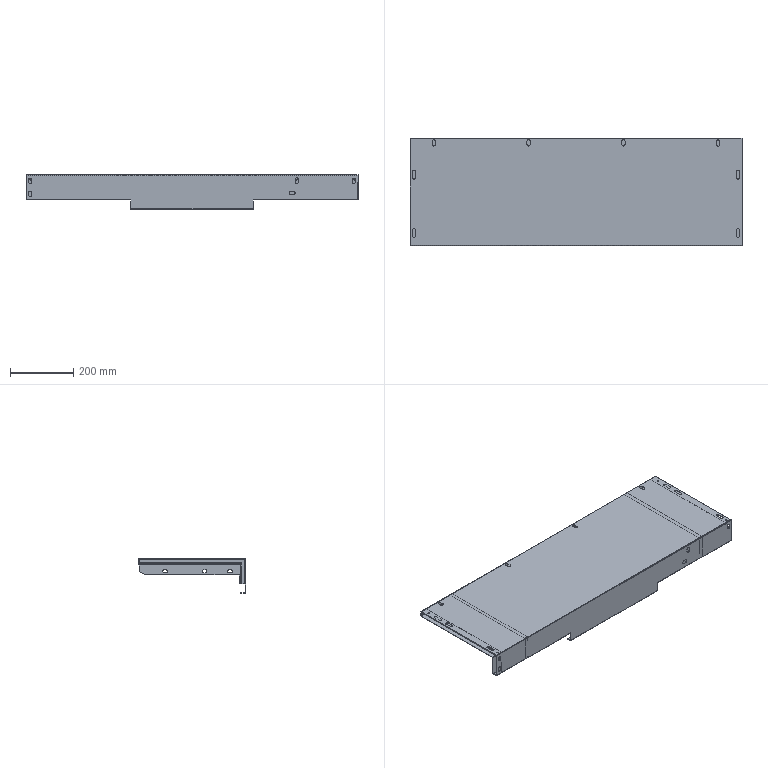Part | SolidWorks | 6 solids | 379 faces | box 1050 x 339.8 x 110 mm | volume 1233242 mm3 | plane 248 | cylinder 131 | commonest cylinder face diameters 6 x48 10 x34 9 x20 0.4 x10 2.4 x5 3.4 x5